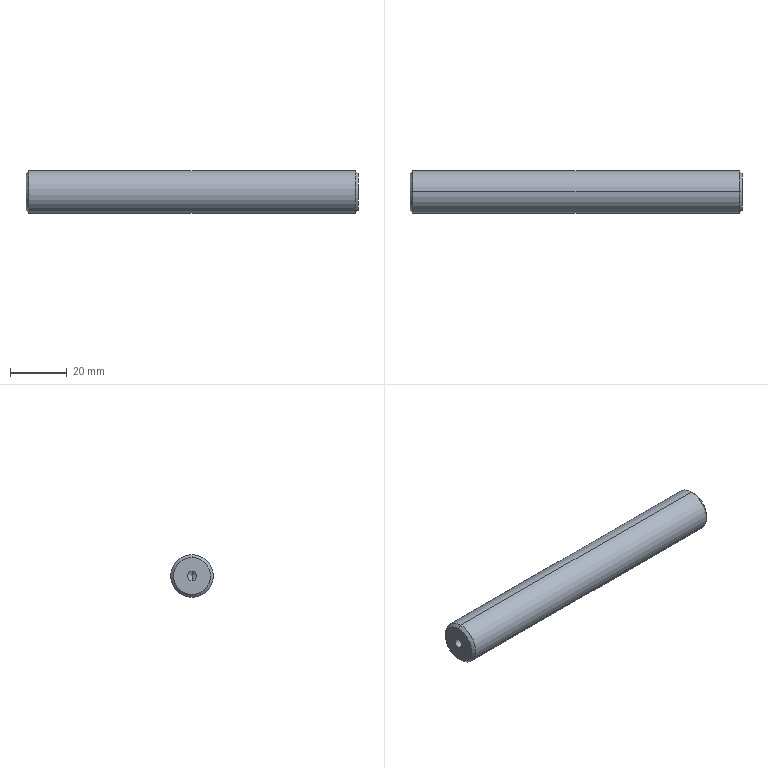Part | SolidWorks | features HoleWzd 2, Chamfer 1, Extrusion 1 | 1 solid | 16 faces | box 117 x 15 x 15 mm | volume 20237 mm3 | cone 8 | cylinder 6 | plane 2 | commonest cylinder face diameters 3.3 x2 5 x2 15 x2
STEP:
#1=CARTESIAN_POINT('',(117.,0.,-6.5));
#2=VERTEX_POINT('',#1);
#3=CARTESIAN_POINT('',(117.,0.,6.5));
#4=VERTEX_POINT('',#3);
#5=CARTESIAN_POINT('',(117.,0.,0.));
#6=DIRECTION('',(1.,0.,0.));
#7=DIRECTION('',(0.,0.,-1.));
#8=AXIS2_PLACEMENT_3D('',#5,#6,#7);
#9=CIRCLE('',#8,6.5);
#10=EDGE_CURVE('',#2,#4,#9,.T.);
#11=ORIENTED_EDGE('',*,*,#10,.F.);
#12=CARTESIAN_POINT('',(116.,0.,-7.5));
#13=VERTEX_POINT('',#12);
#14=CARTESIAN_POINT('',(117.,0.,-6.5));
#15=DIRECTION('',(-0.7071,0.,-0.7071));
#16=VECTOR('',#15,1000.);
#17=LINE('',#14,#16);
#18=EDGE_CURVE('',#2,#13,#17,.T.);
#19=ORIENTED_EDGE('',*,*,#18,.T.);
#20=CARTESIAN_POINT('',(116.,0.,7.5));
#21=VERTEX_POINT('',#20);
#22=CARTESIAN_POINT('',(116.,0.,0.));
#23=DIRECTION('',(-1.,0.,0.));
#24=DIRECTION('',(0.,0.,-1.));
#25=AXIS2_PLACEMENT_3D('',#22,#23,#24);
#26=CIRCLE('',#25,7.5);
#27=EDGE_CURVE('',#21,#13,#26,.T.);
#28=ORIENTED_EDGE('',*,*,#27,.F.);
#29=CARTESIAN_POINT('',(117.,0.,6.5));
#30=DIRECTION('',(-0.7071,0.,0.7071));
#31=VECTOR('',#30,1000.);
#32=LINE('',#29,#31);
#33=EDGE_CURVE('',#4,#21,#32,.T.);
#34=ORIENTED_EDGE('',*,*,#33,.F.);
#35=EDGE_LOOP('',(#11,#19,#28,#34));
#36=FACE_OUTER_BOUND('',#35,.T.);
#37=CARTESIAN_POINT('',(117.,0.,0.));
#38=DIRECTION('',(-1.,0.,0.));
#39=DIRECTION('',(0.,0.,1.));
#40=AXIS2_PLACEMENT_3D('',#37,#38,#39);
#41=CONICAL_SURFACE('',#40,6.5,0.7854);
#42=ADVANCED_FACE('',(#36),#41,.T.);
#43=CARTESIAN_POINT('',(0.,0.,6.5));
#44=VERTEX_POINT('',#43);
#45=CARTESIAN_POINT('',(0.,0.,-6.5));
#46=VERTEX_POINT('',#45);
#47=CARTESIAN_POINT('',(0.,0.,0.));
#48=DIRECTION('',(-1.,0.,0.));
#49=DIRECTION('',(0.,0.,-1.));
#50=AXIS2_PLACEMENT_3D('',#47,#48,#49);
#51=CIRCLE('',#50,6.5);
#52=EDGE_CURVE('',#44,#46,#51,.T.);
#53=ORIENTED_EDGE('',*,*,#52,.F.);
#54=CARTESIAN_POINT('',(1.,0.,7.5));
#55=VERTEX_POINT('',#54);
#56=CARTESIAN_POINT('',(1.,0.,7.5));
#57=DIRECTION('',(0.7071,0.,0.7071));
#58=VECTOR('',#57,1000.);
#59=LINE('',#56,#58);
#60=EDGE_CURVE('',#44,#55,#59,.T.);
#61=ORIENTED_EDGE('',*,*,#60,.T.);
#62=CARTESIAN_POINT('',(1.,0.,-7.5));
#63=VERTEX_POINT('',#62);
#64=CARTESIAN_POINT('',(1.,0.,0.));
#65=DIRECTION('',(1.,0.,0.));
#66=DIRECTION('',(0.,0.,-1.));
#67=AXIS2_PLACEMENT_3D('',#64,#65,#66);
#68=CIRCLE('',#67,7.5);
#69=EDGE_CURVE('',#63,#55,#68,.T.);
#70=ORIENTED_EDGE('',*,*,#69,.F.);
#71=CARTESIAN_POINT('',(1.,0.,-7.5));
#72=DIRECTION('',(0.7071,0.,-0.7071));
#73=VECTOR('',#72,1000.);
#74=LINE('',#71,#73);
#75=EDGE_CURVE('',#46,#63,#74,.T.);
#76=ORIENTED_EDGE('',*,*,#75,.F.);
#77=EDGE_LOOP('',(#53,#61,#70,#76));
#78=FACE_OUTER_BOUND('',#77,.T.);
#79=CARTESIAN_POINT('',(1.,0.,0.));
#80=DIRECTION('',(1.,0.,0.));
#81=DIRECTION('',(0.,0.,-1.));
#82=AXIS2_PLACEMENT_3D('',#79,#80,#81);
#83=CONICAL_SURFACE('',#82,7.5,0.7854);
#84=ADVANCED_FACE('',(#78),#83,.T.);
#85=CARTESIAN_POINT('',(102.,0.,2.5));
#86=VERTEX_POINT('',#85);
#87=CARTESIAN_POINT('',(102.,0.,-2.5));
#88=VERTEX_POINT('',#87);
#89=CARTESIAN_POINT('',(102.,0.,0.));
#90=DIRECTION('',(1.,0.,0.));
#91=DIRECTION('',(0.,0.,-1.));
#92=AXIS2_PLACEMENT_3D('',#89,#90,#91);
#93=CIRCLE('',#92,2.5);
#94=EDGE_CURVE('',#86,#88,#93,.T.);
#95=ORIENTED_EDGE('',*,*,#94,.F.);
#96=CARTESIAN_POINT('',(117.,0.,2.5));
#97=VERTEX_POINT('',#96);
#98=CARTESIAN_POINT('',(117.,0.,2.5));
#99=DIRECTION('',(1.,0.,0.));
#100=VECTOR('',#99,1000.);
#101=LINE('',#98,#100);
#102=EDGE_CURVE('',#86,#97,#101,.T.);
#103=ORIENTED_EDGE('',*,*,#102,.T.);
#104=CARTESIAN_POINT('',(117.,0.,-2.5));
#105=VERTEX_POINT('',#104);
#106=CARTESIAN_POINT('',(117.,0.,0.));
#107=DIRECTION('',(1.,0.,0.));
#108=DIRECTION('',(0.,0.,-1.));
#109=AXIS2_PLACEMENT_3D('',#106,#107,#108);
#110=CIRCLE('',#109,2.5);
#111=EDGE_CURVE('',#97,#105,#110,.T.);
#112=ORIENTED_EDGE('',*,*,#111,.T.);
#113=CARTESIAN_POINT('',(117.,0.,-2.5));
#114=DIRECTION('',(1.,0.,0.));
#115=VECTOR('',#114,1000.);
#116=LINE('',#113,#115);
#117=EDGE_CURVE('',#88,#105,#116,.T.);
#118=ORIENTED_EDGE('',*,*,#117,.F.);
#119=EDGE_LOOP('',(#95,#103,#112,#118));
#120=FACE_OUTER_BOUND('',#119,.T.);
#121=CARTESIAN_POINT('',(117.,0.,0.));
#122=DIRECTION('',(1.,0.,0.));
#123=DIRECTION('',(0.,0.,-1.));
#124=AXIS2_PLACEMENT_3D('',#121,#122,#123);
#125=CYLINDRICAL_SURFACE('',#124,2.5);
#126=ADVANCED_FACE('',(#120),#125,.F.);
#127=CARTESIAN_POINT('',(100.498,0.,0.));
#128=VERTEX_POINT('',#127);
#129=CARTESIAN_POINT('',(102.,0.,-2.5));
#130=DIRECTION('',(0.515,0.,-0.8572));
#131=VECTOR('',#130,1000.);
#132=LINE('',#129,#131);
#133=EDGE_CURVE('',#128,#88,#132,.T.);
#134=ORIENTED_EDGE('',*,*,#133,.F.);
#135=CARTESIAN_POINT('',(102.,0.,2.5));
#136=DIRECTION('',(0.515,0.,0.8572));
#137=VECTOR('',#136,1000.);
#138=LINE('',#135,#137);
#139=EDGE_CURVE('',#128,#86,#138,.T.);
#140=ORIENTED_EDGE('',*,*,#139,.T.);
#141=ORIENTED_EDGE('',*,*,#94,.T.);
#142=EDGE_LOOP('',(#134,#140,#141));
#143=FACE_OUTER_BOUND('',#142,.T.);
#144=CARTESIAN_POINT('',(102.,0.,0.));
#145=DIRECTION('',(1.,0.,0.));
#146=DIRECTION('',(0.,0.,-1.));
#147=AXIS2_PLACEMENT_3D('',#144,#145,#146);
#148=CONICAL_SURFACE('',#147,2.5,1.03);
#149=ADVANCED_FACE('',(#143),#148,.F.);
#150=CARTESIAN_POINT('',(10.1,0.,-1.65));
#151=VERTEX_POINT('',#150);
#152=CARTESIAN_POINT('',(10.1,0.,1.65));
#153=VERTEX_POINT('',#152);
#154=CARTESIAN_POINT('',(10.1,0.,0.));
#155=DIRECTION('',(-1.,0.,0.));
#156=DIRECTION('',(0.,0.,1.));
#157=AXIS2_PLACEMENT_3D('',#154,#155,#156);
#158=CIRCLE('',#157,1.65);
#159=EDGE_CURVE('',#151,#153,#158,.T.);
#160=ORIENTED_EDGE('',*,*,#159,.F.);
#161=CARTESIAN_POINT('',(0.,0.,-1.65));
#162=VERTEX_POINT('',#161);
#163=CARTESIAN_POINT('',(0.,0.,-1.65));
#164=DIRECTION('',(-1.,0.,0.));
#165=VECTOR('',#164,1000.);
#166=LINE('',#163,#165);
#167=EDGE_CURVE('',#151,#162,#166,.T.);
#168=ORIENTED_EDGE('',*,*,#167,.T.);
#169=CARTESIAN_POINT('',(0.,0.,1.65));
#170=VERTEX_POINT('',#169);
#171=CARTESIAN_POINT('',(0.,0.,0.));
#172=DIRECTION('',(-1.,0.,0.));
#173=DIRECTION('',(0.,0.,1.));
#174=AXIS2_PLACEMENT_3D('',#171,#172,#173);
#175=CIRCLE('',#174,1.65);
#176=EDGE_CURVE('',#162,#170,#175,.T.);
#177=ORIENTED_EDGE('',*,*,#176,.T.);
#178=CARTESIAN_POINT('',(0.,0.,1.65));
#179=DIRECTION('',(-1.,0.,0.));
#180=VECTOR('',#179,1000.);
#181=LINE('',#178,#180);
#182=EDGE_CURVE('',#153,#170,#181,.T.);
#183=ORIENTED_EDGE('',*,*,#182,.F.);
#184=EDGE_LOOP('',(#160,#168,#177,#183));
#185=FACE_OUTER_BOUND('',#184,.T.);
#186=CARTESIAN_POINT('',(0.,0.,0.));
#187=DIRECTION('',(-1.,0.,0.));
#188=DIRECTION('',(0.,0.,1.));
#189=AXIS2_PLACEMENT_3D('',#186,#187,#188);
#190=CYLINDRICAL_SURFACE('',#189,1.65);
#191=ADVANCED_FACE('',(#185),#190,.F.);
#192=CARTESIAN_POINT('',(11.091,0.,0.));
#193=VERTEX_POINT('',#192);
#194=CARTESIAN_POINT('',(10.1,0.,1.65));
#195=DIRECTION('',(-0.515,0.,0.8572));
#196=VECTOR('',#195,1000.);
#197=LINE('',#194,#196);
#198=EDGE_CURVE('',#193,#153,#197,.T.);
#199=ORIENTED_EDGE('',*,*,#198,.F.);
#200=CARTESIAN_POINT('',(10.1,0.,-1.65));
#201=DIRECTION('',(-0.515,0.,-0.8572));
#202=VECTOR('',#201,1000.);
#203=LINE('',#200,#202);
#204=EDGE_CURVE('',#193,#151,#203,.T.);
#205=ORIENTED_EDGE('',*,*,#204,.T.);
#206=ORIENTED_EDGE('',*,*,#159,.T.);
#207=EDGE_LOOP('',(#199,#205,#206));
#208=FACE_OUTER_BOUND('',#207,.T.);
#209=CARTESIAN_POINT('',(10.1,0.,0.));
#210=DIRECTION('',(-1.,0.,0.));
#211=DIRECTION('',(0.,0.,1.));
#212=AXIS2_PLACEMENT_3D('',#209,#210,#211);
#213=CONICAL_SURFACE('',#212,1.65,1.03);
#214=ADVANCED_FACE('',(#208),#213,.F.);
#215=ORIENTED_EDGE('',*,*,#27,.T.);
#216=CARTESIAN_POINT('',(117.,0.,-7.5));
#217=DIRECTION('',(-1.,0.,0.));
#218=VECTOR('',#217,1000.);
#219=LINE('',#216,#218);
#220=EDGE_CURVE('',#13,#63,#219,.T.);
#221=ORIENTED_EDGE('',*,*,#220,.T.);
#222=ORIENTED_EDGE('',*,*,#69,.T.);
#223=CARTESIAN_POINT('',(117.,0.,7.5));
#224=DIRECTION('',(-1.,0.,0.));
#225=VECTOR('',#224,1000.);
#226=LINE('',#223,#225);
#227=EDGE_CURVE('',#21,#55,#226,.T.);
#228=ORIENTED_EDGE('',*,*,#227,.F.);
#229=EDGE_LOOP('',(#215,#221,#222,#228));
#230=FACE_OUTER_BOUND('',#229,.T.);
#231=CARTESIAN_POINT('',(117.,0.,0.));
#232=DIRECTION('',(-1.,0.,0.));
#233=DIRECTION('',(0.,0.,1.));
#234=AXIS2_PLACEMENT_3D('',#231,#232,#233);
#235=CYLINDRICAL_SURFACE('',#234,7.5);
#236=ADVANCED_FACE('',(#230),#235,.T.);
#237=ORIENTED_EDGE('',*,*,#220,.F.);
#238=CARTESIAN_POINT('',(116.,0.,0.));
#239=DIRECTION('',(-1.,0.,0.));
#240=DIRECTION('',(0.,0.,-1.));
#241=AXIS2_PLACEMENT_3D('',#238,#239,#240);
#242=CIRCLE('',#241,7.5);
#243=EDGE_CURVE('',#13,#21,#242,.T.);
#244=ORIENTED_EDGE('',*,*,#243,.T.);
#245=ORIENTED_EDGE('',*,*,#227,.T.);
#246=CARTESIAN_POINT('',(1.,0.,0.));
#247=DIRECTION('',(1.,0.,0.));
#248=DIRECTION('',(0.,0.,-1.));
#249=AXIS2_PLACEMENT_3D('',#246,#247,#248);
#250=CIRCLE('',#249,7.5);
#251=EDGE_CURVE('',#55,#63,#250,.T.);
#252=ORIENTED_EDGE('',*,*,#251,.T.);
#253=EDGE_LOOP('',(#237,#244,#245,#252));
#254=FACE_OUTER_BOUND('',#253,.T.);
#255=CARTESIAN_POINT('',(117.,0.,0.));
#256=DIRECTION('',(-1.,0.,0.));
#257=DIRECTION('',(0.,0.,1.));
#258=AXIS2_PLACEMENT_3D('',#255,#256,#257);
#259=CYLINDRICAL_SURFACE('',#258,7.5);
#260=ADVANCED_FACE('',(#254),#259,.T.);
#261=CARTESIAN_POINT('',(117.,0.,0.));
#262=DIRECTION('',(1.,0.,0.));
#263=DIRECTION('',(0.,0.,-1.));
#264=AXIS2_PLACEMENT_3D('',#261,#262,#263);
#265=CIRCLE('',#264,6.5);
#266=EDGE_CURVE('',#4,#2,#265,.T.);
#267=ORIENTED_EDGE('',*,*,#266,.T.);
#268=ORIENTED_EDGE('',*,*,#10,.T.);
#269=EDGE_LOOP('',(#267,#268));
#270=FACE_OUTER_BOUND('',#269,.T.);
#271=CARTESIAN_POINT('',(117.,0.,0.));
#272=DIRECTION('',(1.,0.,0.));
#273=DIRECTION('',(0.,0.,-1.));
#274=AXIS2_PLACEMENT_3D('',#271,#272,#273);
#275=CIRCLE('',#274,2.5);
#276=EDGE_CURVE('',#105,#97,#275,.T.);
#277=ORIENTED_EDGE('',*,*,#276,.F.);
#278=ORIENTED_EDGE('',*,*,#111,.F.);
#279=EDGE_LOOP('',(#277,#278));
#280=FACE_BOUND('',#279,.T.);
#281=CARTESIAN_POINT('',(117.,0.,0.));
#282=DIRECTION('',(1.,0.,0.));
#283=DIRECTION('',(0.,0.,-1.));
#284=AXIS2_PLACEMENT_3D('',#281,#282,#283);
#285=PLANE('',#284);
#286=ADVANCED_FACE('',(#270,#280),#285,.T.);
#287=CARTESIAN_POINT('',(0.,0.,0.));
#288=DIRECTION('',(-1.,0.,0.));
#289=DIRECTION('',(0.,0.,-1.));
#290=AXIS2_PLACEMENT_3D('',#287,#288,#289);
#291=CIRCLE('',#290,6.5);
#292=EDGE_CURVE('',#46,#44,#291,.T.);
#293=ORIENTED_EDGE('',*,*,#292,.T.);
#294=ORIENTED_EDGE('',*,*,#52,.T.);
#295=EDGE_LOOP('',(#293,#294));
#296=FACE_OUTER_BOUND('',#295,.T.);
#297=CARTESIAN_POINT('',(0.,0.,0.));
#298=DIRECTION('',(-1.,0.,0.));
#299=DIRECTION('',(0.,0.,1.));
#300=AXIS2_PLACEMENT_3D('',#297,#298,#299);
#301=CIRCLE('',#300,1.65);
#302=EDGE_CURVE('',#170,#162,#301,.T.);
#303=ORIENTED_EDGE('',*,*,#302,.F.);
#304=ORIENTED_EDGE('',*,*,#176,.F.);
#305=EDGE_LOOP('',(#303,#304));
#306=FACE_BOUND('',#305,.T.);
#307=CARTESIAN_POINT('',(0.,0.,0.));
#308=DIRECTION('',(1.,0.,0.));
#309=DIRECTION('',(0.,0.,-1.));
#310=AXIS2_PLACEMENT_3D('',#307,#308,#309);
#311=PLANE('',#310);
#312=ADVANCED_FACE('',(#296,#306),#311,.F.);
#313=ORIENTED_EDGE('',*,*,#204,.F.);
#314=ORIENTED_EDGE('',*,*,#198,.T.);
#315=CARTESIAN_POINT('',(10.1,0.,0.));
#316=DIRECTION('',(-1.,0.,0.));
#317=DIRECTION('',(0.,0.,1.));
#318=AXIS2_PLACEMENT_3D('',#315,#316,#317);
#319=CIRCLE('',#318,1.65);
#320=EDGE_CURVE('',#153,#151,#319,.T.);
#321=ORIENTED_EDGE('',*,*,#320,.T.);
#322=EDGE_LOOP('',(#313,#314,#321));
#323=FACE_OUTER_BOUND('',#322,.T.);
#324=CARTESIAN_POINT('',(10.1,0.,0.));
#325=DIRECTION('',(-1.,0.,0.));
#326=DIRECTION('',(0.,0.,1.));
#327=AXIS2_PLACEMENT_3D('',#324,#325,#326);
#328=CONICAL_SURFACE('',#327,1.65,1.03);
#329=ADVANCED_FACE('',(#323),#328,.F.);
#330=ORIENTED_EDGE('',*,*,#167,.F.);
#331=ORIENTED_EDGE('',*,*,#320,.F.);
#332=ORIENTED_EDGE('',*,*,#182,.T.);
#333=ORIENTED_EDGE('',*,*,#302,.T.);
#334=EDGE_LOOP('',(#330,#331,#332,#333));
#335=FACE_OUTER_BOUND('',#334,.T.);
#336=CARTESIAN_POINT('',(0.,0.,0.));
#337=DIRECTION('',(-1.,0.,0.));
#338=DIRECTION('',(0.,0.,1.));
#339=AXIS2_PLACEMENT_3D('',#336,#337,#338);
#340=CYLINDRICAL_SURFACE('',#339,1.65);
#341=ADVANCED_FACE('',(#335),#340,.F.);
#342=ORIENTED_EDGE('',*,*,#139,.F.);
#343=ORIENTED_EDGE('',*,*,#133,.T.);
#344=CARTESIAN_POINT('',(102.,0.,0.));
#345=DIRECTION('',(1.,0.,0.));
#346=DIRECTION('',(0.,0.,-1.));
#347=AXIS2_PLACEMENT_3D('',#344,#345,#346);
#348=CIRCLE('',#347,2.5);
#349=EDGE_CURVE('',#88,#86,#348,.T.);
#350=ORIENTED_EDGE('',*,*,#349,.T.);
#351=EDGE_LOOP('',(#342,#343,#350));
#352=FACE_OUTER_BOUND('',#351,.T.);
#353=CARTESIAN_POINT('',(102.,0.,0.));
#354=DIRECTION('',(1.,0.,0.));
#355=DIRECTION('',(0.,0.,-1.));
#356=AXIS2_PLACEMENT_3D('',#353,#354,#355);
#357=CONICAL_SURFACE('',#356,2.5,1.03);
#358=ADVANCED_FACE('',(#352),#357,.F.);
#359=ORIENTED_EDGE('',*,*,#102,.F.);
#360=ORIENTED_EDGE('',*,*,#349,.F.);
#361=ORIENTED_EDGE('',*,*,#117,.T.);
#362=ORIENTED_EDGE('',*,*,#276,.T.);
#363=EDGE_LOOP('',(#359,#360,#361,#362));
#364=FACE_OUTER_BOUND('',#363,.T.);
#365=CARTESIAN_POINT('',(117.,0.,0.));
#366=DIRECTION('',(1.,0.,0.));
#367=DIRECTION('',(0.,0.,-1.));
#368=AXIS2_PLACEMENT_3D('',#365,#366,#367);
#369=CYLINDRICAL_SURFACE('',#368,2.5);
#370=ADVANCED_FACE('',(#364),#369,.F.);
#371=ORIENTED_EDGE('',*,*,#60,.F.);
#372=ORIENTED_EDGE('',*,*,#292,.F.);
#373=ORIENTED_EDGE('',*,*,#75,.T.);
#374=ORIENTED_EDGE('',*,*,#251,.F.);
#375=EDGE_LOOP('',(#371,#372,#373,#374));
#376=FACE_OUTER_BOUND('',#375,.T.);
#377=CARTESIAN_POINT('',(1.,0.,0.));
#378=DIRECTION('',(1.,0.,0.));
#379=DIRECTION('',(0.,0.,-1.));
#380=AXIS2_PLACEMENT_3D('',#377,#378,#379);
#381=CONICAL_SURFACE('',#380,7.5,0.7854);
#382=ADVANCED_FACE('',(#376),#381,.T.);
#383=ORIENTED_EDGE('',*,*,#18,.F.);
#384=ORIENTED_EDGE('',*,*,#266,.F.);
#385=ORIENTED_EDGE('',*,*,#33,.T.);
#386=ORIENTED_EDGE('',*,*,#243,.F.);
#387=EDGE_LOOP('',(#383,#384,#385,#386));
#388=FACE_OUTER_BOUND('',#387,.T.);
#389=CARTESIAN_POINT('',(117.,0.,0.));
#390=DIRECTION('',(-1.,0.,0.));
#391=DIRECTION('',(0.,0.,1.));
#392=AXIS2_PLACEMENT_3D('',#389,#390,#391);
#393=CONICAL_SURFACE('',#392,6.5,0.7854);
#394=ADVANCED_FACE('',(#388),#393,.T.);
#395=CLOSED_SHELL('',(#42,#84,#126,#149,#191,#214,#236,#260,#286,#312,#329,#341,#358,#370,#382,#394));
#396=MANIFOLD_SOLID_BREP('',#395);
#397=CARTESIAN_POINT('',(0.,0.,0.));
#398=DIRECTION('',(0.,0.,1.));
#399=DIRECTION('',(1.,0.,0.));
#400=AXIS2_PLACEMENT_3D('',#397,#398,#399);
#401=(LENGTH_UNIT()NAMED_UNIT(*)SI_UNIT(.MILLI.,.METRE.));
#402=UNCERTAINTY_MEASURE_WITH_UNIT(LENGTH_MEASURE(0.00001),#401,'','');
#403=(NAMED_UNIT(*)PLANE_ANGLE_UNIT()SI_UNIT($,.RADIAN.));
#404=(NAMED_UNIT(*)SI_UNIT($,.STERADIAN.)SOLID_ANGLE_UNIT());
#405=(GEOMETRIC_REPRESENTATION_CONTEXT(3)GLOBAL_UNCERTAINTY_ASSIGNED_CONTEXT((#402))GLOBAL_UNIT_ASSIGNED_CONTEXT((#401,#403,#404))REPRESENTATION_CONTEXT('',''));
#406=ADVANCED_BREP_SHAPE_REPRESENTATION('',(#396,#400),#405);